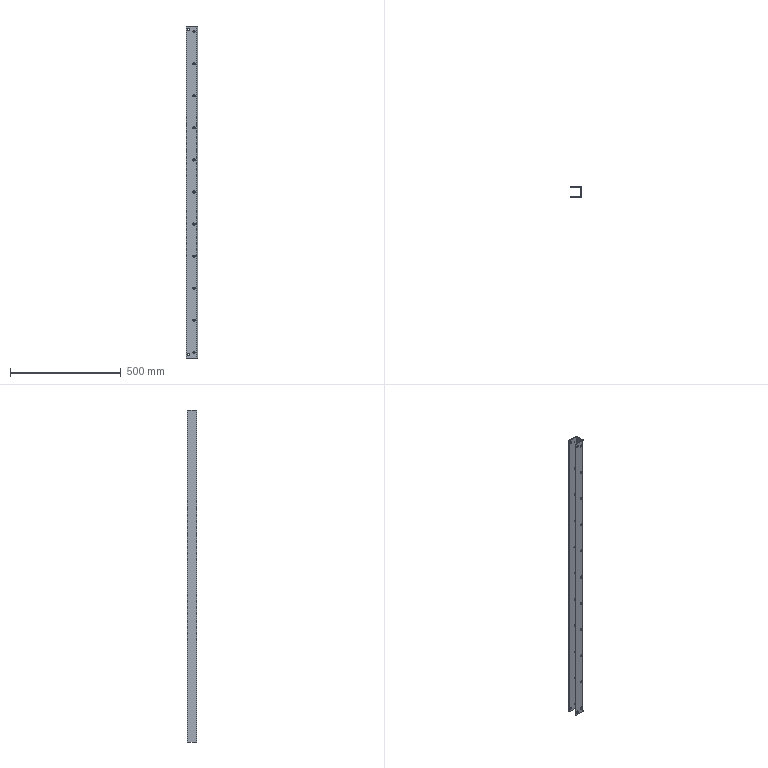Part | NX | features BREP 1 | 1 solid | 66 faces | box 50 x 45 x 1500 mm | volume 511664 mm3 | cylinder 56 | plane 10 | commonest cylinder face diameters 5.5 x22 10 x22 10.5 x8 2 x2 8 x2